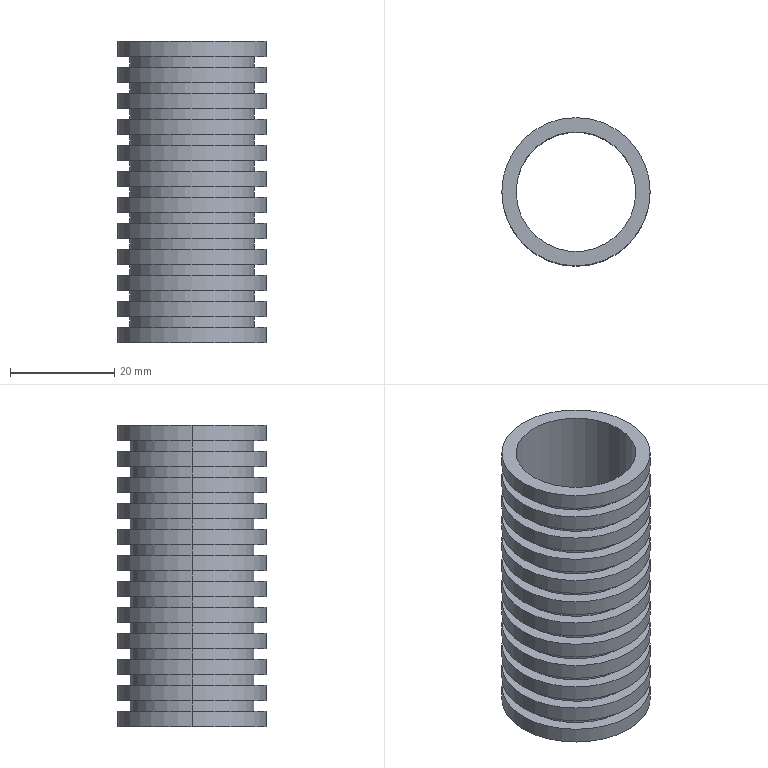Part | STEP file | P0177567_EZT_SCHUTZSCHLAUCH_MKR-23-PG-21.1 | 1 solid | 72 faces | box 28.5 x 28.5 x 58 mm | volume 8821 mm3 | cylinder 48 | plane 24 | commonest cylinder face diameters 28.5 x24 24 x22 23 x2